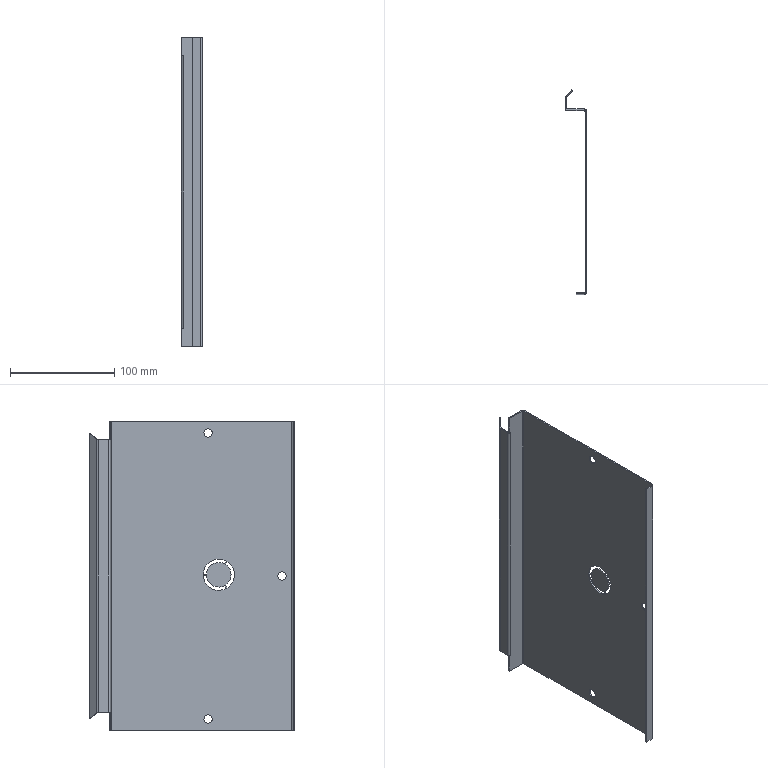Part | SolidWorks | features Attribute 55, Cut 2, SMBaseFlange 2, FlatPattern 1, ICE 1, LibraryFeature 1, MirrorPattern 1, SheetMetal 1 | 1 solid | 66 faces | box 20.2 x 196.571 x 297.6 mm | volume 78731 mm3 | plane 42 | cylinder 22 | spline 2 | commonest cylinder face diameters 8 x6 2 x4 4.4 x4 23.6 x4 30 x4